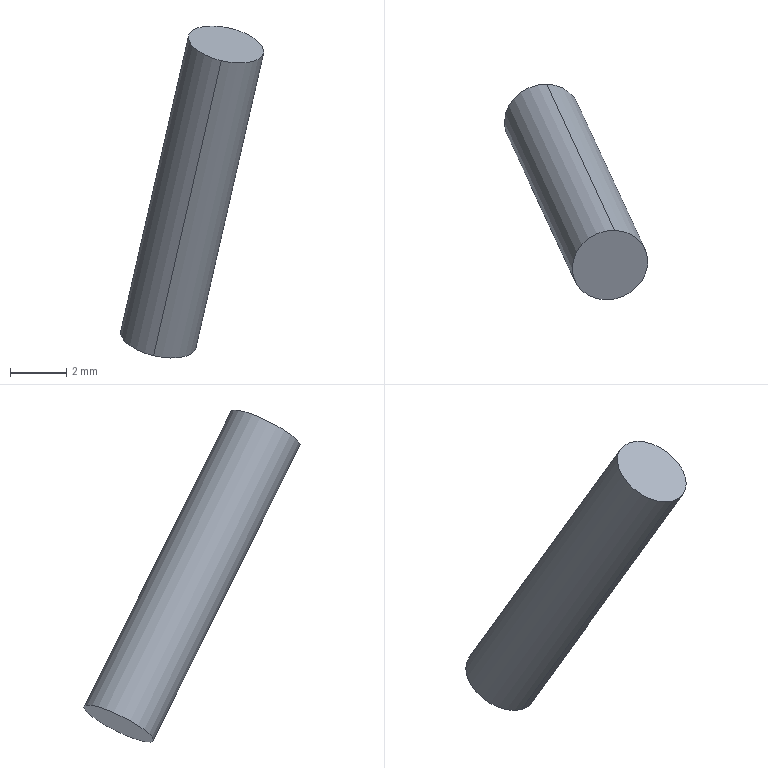Part | SolidWorks | features BaseBody 1 | 1 solid | 5 faces | box 5.111 x 7.707 x 11.846 mm | volume 71.275 mm3 | cylinder 3 | plane 2 | commonest cylinder face diameters 2.75 x3
STEP:
#1=CARTESIAN_POINT('',(1952.591,-179.542,891.979));
#2=VERTEX_POINT('',#1);
#3=CARTESIAN_POINT('',(1951.085,-180.779,891.71));
#4=VERTEX_POINT('',#3);
#5=CARTESIAN_POINT('',(1951.251,-179.542,892.287));
#6=DIRECTION('',(-0.2015,0.436,-0.8771));
#7=DIRECTION('',(0.1206,0.8997,0.4195));
#8=AXIS2_PLACEMENT_3D('',#5,#6,#7);
#9=CIRCLE('',#8,1.375);
#10=EDGE_CURVE('',#2,#4,#9,.T.);
#11=ORIENTED_EDGE('',*,*,#10,.F.);
#12=CARTESIAN_POINT('',(1955.008,-184.774,902.504));
#13=VERTEX_POINT('',#12);
#14=CARTESIAN_POINT('',(1952.542,-179.437,891.768));
#15=DIRECTION('',(0.2015,-0.436,0.8771));
#16=VECTOR('',#15,1000.);
#17=LINE('',#14,#16);
#18=EDGE_CURVE('',#2,#13,#17,.T.);
#19=ORIENTED_EDGE('',*,*,#18,.T.);
#20=CARTESIAN_POINT('',(1953.502,-186.011,902.235));
#21=VERTEX_POINT('',#20);
#22=CARTESIAN_POINT('',(1953.668,-184.774,902.812));
#23=DIRECTION('',(-0.2015,0.436,-0.8771));
#24=DIRECTION('',(-0.09761,-0.8999,-0.425));
#25=AXIS2_PLACEMENT_3D('',#22,#23,#24);
#26=CIRCLE('',#25,1.375);
#27=EDGE_CURVE('',#13,#21,#26,.T.);
#28=ORIENTED_EDGE('',*,*,#27,.T.);
#29=CARTESIAN_POINT('',(1951.085,-180.779,891.71));
#30=DIRECTION('',(0.2015,-0.436,0.8771));
#31=VECTOR('',#30,1000.);
#32=LINE('',#29,#31);
#33=EDGE_CURVE('',#4,#21,#32,.T.);
#34=ORIENTED_EDGE('',*,*,#33,.F.);
#35=EDGE_LOOP('',(#11,#19,#28,#34));
#36=FACE_OUTER_BOUND('',#35,.T.);
#37=CARTESIAN_POINT('',(1951.202,-179.437,892.076));
#38=DIRECTION('',(0.2015,-0.436,0.8771));
#39=DIRECTION('',(0.9746,0.,-0.2239));
#40=AXIS2_PLACEMENT_3D('',#37,#38,#39);
#41=CYLINDRICAL_SURFACE('',#40,1.375);
#42=ADVANCED_FACE('',(#36),#41,.T.);
#43=CARTESIAN_POINT('',(1953.834,-183.537,903.389));
#44=VERTEX_POINT('',#43);
#45=CARTESIAN_POINT('',(1951.416,-178.305,892.864));
#46=VERTEX_POINT('',#45);
#47=CARTESIAN_POINT('',(1951.416,-178.305,892.864));
#48=DIRECTION('',(-0.2015,0.436,-0.8771));
#49=VECTOR('',#48,1000.);
#50=LINE('',#47,#49);
#51=EDGE_CURVE('',#44,#46,#50,.T.);
#52=ORIENTED_EDGE('',*,*,#51,.T.);
#53=CARTESIAN_POINT('',(1951.251,-179.542,892.287));
#54=DIRECTION('',(-0.2015,0.436,-0.8771));
#55=DIRECTION('',(-0.1206,-0.8997,-0.4195));
#56=AXIS2_PLACEMENT_3D('',#53,#54,#55);
#57=CIRCLE('',#56,1.375);
#58=EDGE_CURVE('',#4,#46,#57,.T.);
#59=ORIENTED_EDGE('',*,*,#58,.F.);
#60=ORIENTED_EDGE('',*,*,#33,.T.);
#61=CARTESIAN_POINT('',(1953.668,-184.774,902.812));
#62=DIRECTION('',(0.2015,-0.436,0.8771));
#63=DIRECTION('',(0.1206,0.8997,0.4195));
#64=AXIS2_PLACEMENT_3D('',#61,#62,#63);
#65=CIRCLE('',#64,1.375);
#66=EDGE_CURVE('',#44,#21,#65,.T.);
#67=ORIENTED_EDGE('',*,*,#66,.F.);
#68=EDGE_LOOP('',(#52,#59,#60,#67));
#69=FACE_OUTER_BOUND('',#68,.T.);
#70=CARTESIAN_POINT('',(1951.202,-179.437,892.076));
#71=DIRECTION('',(0.2015,-0.436,0.8771));
#72=DIRECTION('',(-0.09761,-0.8999,-0.425));
#73=AXIS2_PLACEMENT_3D('',#70,#71,#72);
#74=CYLINDRICAL_SURFACE('',#73,1.375);
#75=ADVANCED_FACE('',(#69),#74,.T.);
#76=ORIENTED_EDGE('',*,*,#66,.T.);
#77=ORIENTED_EDGE('',*,*,#27,.F.);
#78=CARTESIAN_POINT('',(1953.668,-184.774,902.812));
#79=DIRECTION('',(-0.2015,0.436,-0.8771));
#80=DIRECTION('',(-0.09761,-0.8999,-0.425));
#81=AXIS2_PLACEMENT_3D('',#78,#79,#80);
#82=CIRCLE('',#81,1.375);
#83=EDGE_CURVE('',#44,#13,#82,.T.);
#84=ORIENTED_EDGE('',*,*,#83,.F.);
#85=EDGE_LOOP('',(#76,#77,#84));
#86=FACE_OUTER_BOUND('',#85,.T.);
#87=CARTESIAN_POINT('',(1954.927,-186.065,901.881));
#88=DIRECTION('',(0.2015,-0.436,0.8771));
#89=DIRECTION('',(0.09761,0.8999,0.425));
#90=AXIS2_PLACEMENT_3D('',#87,#88,#89);
#91=PLANE('',#90);
#92=ADVANCED_FACE('',(#86),#91,.T.);
#93=ORIENTED_EDGE('',*,*,#18,.F.);
#94=CARTESIAN_POINT('',(1951.251,-179.542,892.287));
#95=DIRECTION('',(-0.2015,0.436,-0.8771));
#96=DIRECTION('',(0.1206,0.8997,0.4195));
#97=AXIS2_PLACEMENT_3D('',#94,#95,#96);
#98=CIRCLE('',#97,1.375);
#99=EDGE_CURVE('',#46,#2,#98,.T.);
#100=ORIENTED_EDGE('',*,*,#99,.F.);
#101=ORIENTED_EDGE('',*,*,#51,.F.);
#102=ORIENTED_EDGE('',*,*,#83,.T.);
#103=EDGE_LOOP('',(#93,#100,#101,#102));
#104=FACE_OUTER_BOUND('',#103,.T.);
#105=CARTESIAN_POINT('',(1951.202,-179.437,892.076));
#106=DIRECTION('',(0.2015,-0.436,0.8771));
#107=DIRECTION('',(0.9746,0.,-0.2239));
#108=AXIS2_PLACEMENT_3D('',#105,#106,#107);
#109=CYLINDRICAL_SURFACE('',#108,1.375);
#110=ADVANCED_FACE('',(#104),#109,.T.);
#111=ORIENTED_EDGE('',*,*,#99,.T.);
#112=ORIENTED_EDGE('',*,*,#10,.T.);
#113=ORIENTED_EDGE('',*,*,#58,.T.);
#114=EDGE_LOOP('',(#111,#112,#113));
#115=FACE_OUTER_BOUND('',#114,.T.);
#116=CARTESIAN_POINT('',(1952.509,-180.833,891.356));
#117=DIRECTION('',(-0.2015,0.436,-0.8771));
#118=DIRECTION('',(-0.9746,0.,0.2239));
#119=AXIS2_PLACEMENT_3D('',#116,#117,#118);
#120=PLANE('',#119);
#121=ADVANCED_FACE('',(#115),#120,.T.);
#122=CLOSED_SHELL('',(#42,#75,#92,#110,#121));
#123=MANIFOLD_SOLID_BREP('',#122);
#124=CARTESIAN_POINT('',(0.,0.,0.));
#125=DIRECTION('',(0.,0.,1.));
#126=DIRECTION('',(1.,0.,0.));
#127=AXIS2_PLACEMENT_3D('',#124,#125,#126);
#128=(LENGTH_UNIT()NAMED_UNIT(*)SI_UNIT(.MILLI.,.METRE.));
#129=UNCERTAINTY_MEASURE_WITH_UNIT(LENGTH_MEASURE(0.00001),#128,'','');
#130=(NAMED_UNIT(*)PLANE_ANGLE_UNIT()SI_UNIT($,.RADIAN.));
#131=(NAMED_UNIT(*)SI_UNIT($,.STERADIAN.)SOLID_ANGLE_UNIT());
#132=(GEOMETRIC_REPRESENTATION_CONTEXT(3)GLOBAL_UNCERTAINTY_ASSIGNED_CONTEXT((#129))GLOBAL_UNIT_ASSIGNED_CONTEXT((#128,#130,#131))REPRESENTATION_CONTEXT('',''));
#133=ADVANCED_BREP_SHAPE_REPRESENTATION('',(#123,#127),#132);